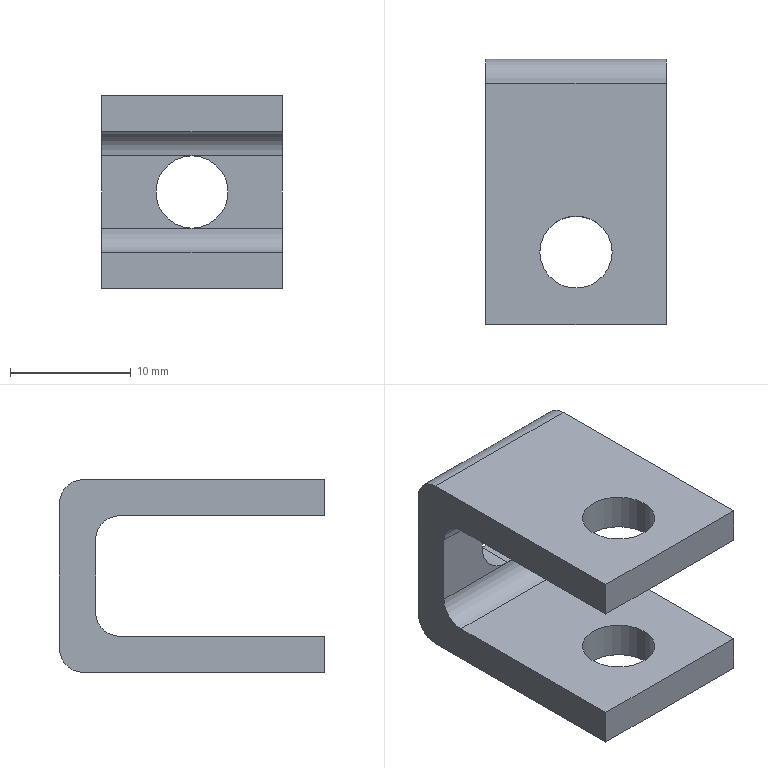Part | SolidWorks | features ICE 2, Extrusion 1, Fillet 1 | 1 solid | 21 faces | box 15 x 22 x 16 mm | volume 2176 mm3 | plane 11 | cylinder 10 | commonest cylinder face diameters 6 x6 4 x4
STEP:
#1=CARTESIAN_POINT('',(0.,13.,-3.));
#2=VERTEX_POINT('',#1);
#3=CARTESIAN_POINT('',(0.,13.,3.));
#4=VERTEX_POINT('',#3);
#5=CARTESIAN_POINT('',(0.,13.,0.));
#6=DIRECTION('',(0.,1.,0.));
#7=DIRECTION('',(0.,0.,1.));
#8=AXIS2_PLACEMENT_3D('',#5,#6,#7);
#9=CIRCLE('',#8,3.);
#10=EDGE_CURVE('',#2,#4,#9,.T.);
#11=ORIENTED_EDGE('',*,*,#10,.F.);
#12=CARTESIAN_POINT('',(0.,16.,-3.));
#13=VERTEX_POINT('',#12);
#14=CARTESIAN_POINT('',(0.,-2.,-3.));
#15=DIRECTION('',(0.,1.,0.));
#16=VECTOR('',#15,1000.);
#17=LINE('',#14,#16);
#18=EDGE_CURVE('',#2,#13,#17,.T.);
#19=ORIENTED_EDGE('',*,*,#18,.T.);
#20=CARTESIAN_POINT('',(0.,16.,3.));
#21=VERTEX_POINT('',#20);
#22=CARTESIAN_POINT('',(0.,16.,0.));
#23=DIRECTION('',(0.,1.,0.));
#24=DIRECTION('',(0.,0.,1.));
#25=AXIS2_PLACEMENT_3D('',#22,#23,#24);
#26=CIRCLE('',#25,3.);
#27=EDGE_CURVE('',#13,#21,#26,.T.);
#28=ORIENTED_EDGE('',*,*,#27,.T.);
#29=CARTESIAN_POINT('',(0.,-2.,3.));
#30=DIRECTION('',(0.,1.,0.));
#31=VECTOR('',#30,1000.);
#32=LINE('',#29,#31);
#33=EDGE_CURVE('',#4,#21,#32,.T.);
#34=ORIENTED_EDGE('',*,*,#33,.F.);
#35=EDGE_LOOP('',(#11,#19,#28,#34));
#36=FACE_OUTER_BOUND('',#35,.T.);
#37=CARTESIAN_POINT('',(0.,-2.,0.));
#38=DIRECTION('',(0.,1.,0.));
#39=DIRECTION('',(0.,0.,1.));
#40=AXIS2_PLACEMENT_3D('',#37,#38,#39);
#41=CYLINDRICAL_SURFACE('',#40,3.);
#42=ADVANCED_FACE('',(#36),#41,.F.);
#43=CARTESIAN_POINT('',(3.,0.,-5.));
#44=VERTEX_POINT('',#43);
#45=CARTESIAN_POINT('',(-3.,0.,-5.));
#46=VERTEX_POINT('',#45);
#47=CARTESIAN_POINT('',(0.,0.,-5.));
#48=DIRECTION('',(0.,0.,-1.));
#49=DIRECTION('',(-1.,0.,0.));
#50=AXIS2_PLACEMENT_3D('',#47,#48,#49);
#51=CIRCLE('',#50,3.);
#52=EDGE_CURVE('',#44,#46,#51,.T.);
#53=ORIENTED_EDGE('',*,*,#52,.F.);
#54=CARTESIAN_POINT('',(3.,0.,-8.));
#55=VERTEX_POINT('',#54);
#56=CARTESIAN_POINT('',(3.,0.,8.));
#57=DIRECTION('',(0.,0.,-1.));
#58=VECTOR('',#57,1000.);
#59=LINE('',#56,#58);
#60=EDGE_CURVE('',#44,#55,#59,.T.);
#61=ORIENTED_EDGE('',*,*,#60,.T.);
#62=CARTESIAN_POINT('',(-3.,0.,-8.));
#63=VERTEX_POINT('',#62);
#64=CARTESIAN_POINT('',(0.,0.,-8.));
#65=DIRECTION('',(0.,0.,1.));
#66=DIRECTION('',(1.,0.,0.));
#67=AXIS2_PLACEMENT_3D('',#64,#65,#66);
#68=CIRCLE('',#67,3.);
#69=EDGE_CURVE('',#63,#55,#68,.T.);
#70=ORIENTED_EDGE('',*,*,#69,.F.);
#71=CARTESIAN_POINT('',(-3.,0.,8.));
#72=DIRECTION('',(0.,0.,-1.));
#73=VECTOR('',#72,1000.);
#74=LINE('',#71,#73);
#75=EDGE_CURVE('',#46,#63,#74,.T.);
#76=ORIENTED_EDGE('',*,*,#75,.F.);
#77=EDGE_LOOP('',(#53,#61,#70,#76));
#78=FACE_OUTER_BOUND('',#77,.T.);
#79=CARTESIAN_POINT('',(0.,0.,8.));
#80=DIRECTION('',(0.,0.,-1.));
#81=DIRECTION('',(-1.,0.,0.));
#82=AXIS2_PLACEMENT_3D('',#79,#80,#81);
#83=CYLINDRICAL_SURFACE('',#82,3.);
#84=ADVANCED_FACE('',(#78),#83,.F.);
#85=CARTESIAN_POINT('',(-3.,0.,8.));
#86=VERTEX_POINT('',#85);
#87=CARTESIAN_POINT('',(3.,0.,8.));
#88=VERTEX_POINT('',#87);
#89=CARTESIAN_POINT('',(0.,0.,8.));
#90=DIRECTION('',(0.,0.,1.));
#91=DIRECTION('',(1.,0.,0.));
#92=AXIS2_PLACEMENT_3D('',#89,#90,#91);
#93=CIRCLE('',#92,3.);
#94=EDGE_CURVE('',#86,#88,#93,.T.);
#95=ORIENTED_EDGE('',*,*,#94,.T.);
#96=CARTESIAN_POINT('',(3.,0.,5.));
#97=VERTEX_POINT('',#96);
#98=CARTESIAN_POINT('',(3.,0.,8.));
#99=DIRECTION('',(0.,0.,-1.));
#100=VECTOR('',#99,1000.);
#101=LINE('',#98,#100);
#102=EDGE_CURVE('',#88,#97,#101,.T.);
#103=ORIENTED_EDGE('',*,*,#102,.T.);
#104=CARTESIAN_POINT('',(-3.,0.,5.));
#105=VERTEX_POINT('',#104);
#106=CARTESIAN_POINT('',(0.,0.,5.));
#107=DIRECTION('',(0.,0.,1.));
#108=DIRECTION('',(1.,0.,0.));
#109=AXIS2_PLACEMENT_3D('',#106,#107,#108);
#110=CIRCLE('',#109,3.);
#111=EDGE_CURVE('',#105,#97,#110,.T.);
#112=ORIENTED_EDGE('',*,*,#111,.F.);
#113=CARTESIAN_POINT('',(-3.,0.,8.));
#114=DIRECTION('',(0.,0.,-1.));
#115=VECTOR('',#114,1000.);
#116=LINE('',#113,#115);
#117=EDGE_CURVE('',#86,#105,#116,.T.);
#118=ORIENTED_EDGE('',*,*,#117,.F.);
#119=EDGE_LOOP('',(#95,#103,#112,#118));
#120=FACE_OUTER_BOUND('',#119,.T.);
#121=CARTESIAN_POINT('',(0.,0.,8.));
#122=DIRECTION('',(0.,0.,-1.));
#123=DIRECTION('',(-1.,0.,0.));
#124=AXIS2_PLACEMENT_3D('',#121,#122,#123);
#125=CYLINDRICAL_SURFACE('',#124,3.);
#126=ADVANCED_FACE('',(#120),#125,.F.);
#127=CARTESIAN_POINT('',(7.5,13.,3.));
#128=VERTEX_POINT('',#127);
#129=CARTESIAN_POINT('',(-7.5,13.,3.));
#130=DIRECTION('',(-1.,0.,0.));
#131=VECTOR('',#130,1000.);
#132=LINE('',#129,#131);
#133=EDGE_CURVE('',#128,#4,#132,.T.);
#134=ORIENTED_EDGE('',*,*,#133,.T.);
#135=CARTESIAN_POINT('',(0.,13.,0.));
#136=DIRECTION('',(0.,1.,0.));
#137=DIRECTION('',(0.,0.,1.));
#138=AXIS2_PLACEMENT_3D('',#135,#136,#137);
#139=CIRCLE('',#138,3.);
#140=EDGE_CURVE('',#4,#2,#139,.T.);
#141=ORIENTED_EDGE('',*,*,#140,.T.);
#142=CARTESIAN_POINT('',(7.5,13.,-3.));
#143=VERTEX_POINT('',#142);
#144=CARTESIAN_POINT('',(7.5,13.,-3.));
#145=DIRECTION('',(1.,0.,0.));
#146=VECTOR('',#145,1000.);
#147=LINE('',#144,#146);
#148=EDGE_CURVE('',#2,#143,#147,.T.);
#149=ORIENTED_EDGE('',*,*,#148,.T.);
#150=CARTESIAN_POINT('',(7.5,13.,5.));
#151=DIRECTION('',(0.,0.,1.));
#152=VECTOR('',#151,1000.);
#153=LINE('',#150,#152);
#154=EDGE_CURVE('',#143,#128,#153,.T.);
#155=ORIENTED_EDGE('',*,*,#154,.T.);
#156=EDGE_LOOP('',(#134,#141,#149,#155));
#157=FACE_OUTER_BOUND('',#156,.T.);
#158=CARTESIAN_POINT('',(-7.5,13.,5.));
#159=DIRECTION('',(0.,1.,0.));
#160=DIRECTION('',(0.,0.,1.));
#161=AXIS2_PLACEMENT_3D('',#158,#159,#160);
#162=PLANE('',#161);
#163=ADVANCED_FACE('',(#157),#162,.F.);
#164=CARTESIAN_POINT('',(-7.5,-6.,8.));
#165=VERTEX_POINT('',#164);
#166=CARTESIAN_POINT('',(-7.5,-6.,5.));
#167=VERTEX_POINT('',#166);
#168=CARTESIAN_POINT('',(-7.5,-6.,8.));
#169=DIRECTION('',(0.,0.,-1.));
#170=VECTOR('',#169,1000.);
#171=LINE('',#168,#170);
#172=EDGE_CURVE('',#165,#167,#171,.T.);
#173=ORIENTED_EDGE('',*,*,#172,.T.);
#174=CARTESIAN_POINT('',(7.5,-6.,5.));
#175=VERTEX_POINT('',#174);
#176=CARTESIAN_POINT('',(-7.5,-6.,5.));
#177=DIRECTION('',(1.,0.,0.));
#178=VECTOR('',#177,1000.);
#179=LINE('',#176,#178);
#180=EDGE_CURVE('',#167,#175,#179,.T.);
#181=ORIENTED_EDGE('',*,*,#180,.T.);
#182=CARTESIAN_POINT('',(7.5,-6.,8.));
#183=VERTEX_POINT('',#182);
#184=CARTESIAN_POINT('',(7.5,-6.,8.));
#185=DIRECTION('',(0.,0.,-1.));
#186=VECTOR('',#185,1000.);
#187=LINE('',#184,#186);
#188=EDGE_CURVE('',#183,#175,#187,.T.);
#189=ORIENTED_EDGE('',*,*,#188,.F.);
#190=CARTESIAN_POINT('',(-7.5,-6.,8.));
#191=DIRECTION('',(1.,0.,0.));
#192=VECTOR('',#191,1000.);
#193=LINE('',#190,#192);
#194=EDGE_CURVE('',#165,#183,#193,.T.);
#195=ORIENTED_EDGE('',*,*,#194,.F.);
#196=EDGE_LOOP('',(#173,#181,#189,#195));
#197=FACE_OUTER_BOUND('',#196,.T.);
#198=CARTESIAN_POINT('',(-7.5,-6.,8.));
#199=DIRECTION('',(0.,1.,0.));
#200=DIRECTION('',(0.,0.,1.));
#201=AXIS2_PLACEMENT_3D('',#198,#199,#200);
#202=PLANE('',#201);
#203=ADVANCED_FACE('',(#197),#202,.F.);
#204=ORIENTED_EDGE('',*,*,#102,.F.);
#205=CARTESIAN_POINT('',(0.,0.,8.));
#206=DIRECTION('',(0.,0.,1.));
#207=DIRECTION('',(1.,0.,0.));
#208=AXIS2_PLACEMENT_3D('',#205,#206,#207);
#209=CIRCLE('',#208,3.);
#210=EDGE_CURVE('',#88,#86,#209,.T.);
#211=ORIENTED_EDGE('',*,*,#210,.T.);
#212=ORIENTED_EDGE('',*,*,#117,.T.);
#213=CARTESIAN_POINT('',(0.,0.,5.));
#214=DIRECTION('',(0.,0.,1.));
#215=DIRECTION('',(1.,0.,0.));
#216=AXIS2_PLACEMENT_3D('',#213,#214,#215);
#217=CIRCLE('',#216,3.);
#218=EDGE_CURVE('',#97,#105,#217,.T.);
#219=ORIENTED_EDGE('',*,*,#218,.F.);
#220=EDGE_LOOP('',(#204,#211,#212,#219));
#221=FACE_OUTER_BOUND('',#220,.T.);
#222=CARTESIAN_POINT('',(0.,0.,8.));
#223=DIRECTION('',(0.,0.,-1.));
#224=DIRECTION('',(-1.,0.,0.));
#225=AXIS2_PLACEMENT_3D('',#222,#223,#224);
#226=CYLINDRICAL_SURFACE('',#225,3.);
#227=ADVANCED_FACE('',(#221),#226,.F.);
#228=CARTESIAN_POINT('',(7.5,14.,8.));
#229=VERTEX_POINT('',#228);
#230=CARTESIAN_POINT('',(7.5,-6.,8.));
#231=DIRECTION('',(0.,1.,0.));
#232=VECTOR('',#231,1000.);
#233=LINE('',#230,#232);
#234=EDGE_CURVE('',#183,#229,#233,.T.);
#235=ORIENTED_EDGE('',*,*,#234,.T.);
#236=CARTESIAN_POINT('',(-7.5,14.,8.));
#237=VERTEX_POINT('',#236);
#238=CARTESIAN_POINT('',(0.,14.,8.));
#239=DIRECTION('',(-1.,0.,0.));
#240=VECTOR('',#239,1000.);
#241=LINE('',#238,#240);
#242=EDGE_CURVE('',#229,#237,#241,.T.);
#243=ORIENTED_EDGE('',*,*,#242,.T.);
#244=CARTESIAN_POINT('',(-7.5,-6.,8.));
#245=DIRECTION('',(0.,-1.,0.));
#246=VECTOR('',#245,1000.);
#247=LINE('',#244,#246);
#248=EDGE_CURVE('',#237,#165,#247,.T.);
#249=ORIENTED_EDGE('',*,*,#248,.T.);
#250=ORIENTED_EDGE('',*,*,#194,.T.);
#251=EDGE_LOOP('',(#235,#243,#249,#250));
#252=FACE_OUTER_BOUND('',#251,.T.);
#253=ORIENTED_EDGE('',*,*,#94,.F.);
#254=ORIENTED_EDGE('',*,*,#210,.F.);
#255=EDGE_LOOP('',(#253,#254));
#256=FACE_BOUND('',#255,.T.);
#257=CARTESIAN_POINT('',(0.,0.,8.));
#258=DIRECTION('',(0.,0.,-1.));
#259=DIRECTION('',(-1.,0.,0.));
#260=AXIS2_PLACEMENT_3D('',#257,#258,#259);
#261=PLANE('',#260);
#262=ADVANCED_FACE('',(#252,#256),#261,.F.);
#263=CARTESIAN_POINT('',(-7.5,14.,-8.));
#264=VERTEX_POINT('',#263);
#265=CARTESIAN_POINT('',(-7.5,-6.,-8.));
#266=VERTEX_POINT('',#265);
#267=CARTESIAN_POINT('',(-7.5,-6.,-8.));
#268=DIRECTION('',(0.,-1.,0.));
#269=VECTOR('',#268,1000.);
#270=LINE('',#267,#269);
#271=EDGE_CURVE('',#264,#266,#270,.T.);
#272=ORIENTED_EDGE('',*,*,#271,.F.);
#273=CARTESIAN_POINT('',(7.5,14.,-8.));
#274=VERTEX_POINT('',#273);
#275=CARTESIAN_POINT('',(7.5,14.,-8.));
#276=DIRECTION('',(1.,0.,0.));
#277=VECTOR('',#276,1000.);
#278=LINE('',#275,#277);
#279=EDGE_CURVE('',#264,#274,#278,.T.);
#280=ORIENTED_EDGE('',*,*,#279,.T.);
#281=CARTESIAN_POINT('',(7.5,-6.,-8.));
#282=VERTEX_POINT('',#281);
#283=CARTESIAN_POINT('',(7.5,-6.,-8.));
#284=DIRECTION('',(0.,1.,0.));
#285=VECTOR('',#284,1000.);
#286=LINE('',#283,#285);
#287=EDGE_CURVE('',#282,#274,#286,.T.);
#288=ORIENTED_EDGE('',*,*,#287,.F.);
#289=CARTESIAN_POINT('',(-7.5,-6.,-8.));
#290=DIRECTION('',(1.,0.,0.));
#291=VECTOR('',#290,1000.);
#292=LINE('',#289,#291);
#293=EDGE_CURVE('',#266,#282,#292,.T.);
#294=ORIENTED_EDGE('',*,*,#293,.F.);
#295=EDGE_LOOP('',(#272,#280,#288,#294));
#296=FACE_OUTER_BOUND('',#295,.T.);
#297=ORIENTED_EDGE('',*,*,#69,.T.);
#298=CARTESIAN_POINT('',(0.,0.,-8.));
#299=DIRECTION('',(0.,0.,1.));
#300=DIRECTION('',(1.,0.,0.));
#301=AXIS2_PLACEMENT_3D('',#298,#299,#300);
#302=CIRCLE('',#301,3.);
#303=EDGE_CURVE('',#55,#63,#302,.T.);
#304=ORIENTED_EDGE('',*,*,#303,.T.);
#305=EDGE_LOOP('',(#297,#304));
#306=FACE_BOUND('',#305,.T.);
#307=CARTESIAN_POINT('',(0.,0.,-8.));
#308=DIRECTION('',(0.,0.,-1.));
#309=DIRECTION('',(-1.,0.,0.));
#310=AXIS2_PLACEMENT_3D('',#307,#308,#309);
#311=PLANE('',#310);
#312=ADVANCED_FACE('',(#296,#306),#311,.T.);
#313=CARTESIAN_POINT('',(-7.5,16.,6.));
#314=VERTEX_POINT('',#313);
#315=CARTESIAN_POINT('',(-7.5,16.,-6.));
#316=VERTEX_POINT('',#315);
#317=CARTESIAN_POINT('',(-7.5,16.,8.));
#318=DIRECTION('',(0.,0.,-1.));
#319=VECTOR('',#318,1000.);
#320=LINE('',#317,#319);
#321=EDGE_CURVE('',#314,#316,#320,.T.);
#322=ORIENTED_EDGE('',*,*,#321,.T.);
#323=CARTESIAN_POINT('',(-7.5,14.,-6.));
#324=DIRECTION('',(-1.,0.,0.));
#325=DIRECTION('',(0.,0.,-1.));
#326=AXIS2_PLACEMENT_3D('',#323,#324,#325);
#327=CIRCLE('',#326,2.);
#328=EDGE_CURVE('',#316,#264,#327,.T.);
#329=ORIENTED_EDGE('',*,*,#328,.T.);
#330=ORIENTED_EDGE('',*,*,#271,.T.);
#331=CARTESIAN_POINT('',(-7.5,-6.,-5.));
#332=VERTEX_POINT('',#331);
#333=CARTESIAN_POINT('',(-7.5,-6.,8.));
#334=DIRECTION('',(0.,0.,-1.));
#335=VECTOR('',#334,1000.);
#336=LINE('',#333,#335);
#337=EDGE_CURVE('',#332,#266,#336,.T.);
#338=ORIENTED_EDGE('',*,*,#337,.F.);
#339=CARTESIAN_POINT('',(-7.5,11.,-5.));
#340=VERTEX_POINT('',#339);
#341=CARTESIAN_POINT('',(-7.5,-6.,-5.));
#342=DIRECTION('',(0.,1.,0.));
#343=VECTOR('',#342,1000.);
#344=LINE('',#341,#343);
#345=EDGE_CURVE('',#332,#340,#344,.T.);
#346=ORIENTED_EDGE('',*,*,#345,.T.);
#347=CARTESIAN_POINT('',(-7.5,13.,-3.));
#348=VERTEX_POINT('',#347);
#349=CARTESIAN_POINT('',(-7.5,11.,-3.));
#350=DIRECTION('',(1.,0.,0.));
#351=DIRECTION('',(0.,0.,-1.));
#352=AXIS2_PLACEMENT_3D('',#349,#350,#351);
#353=CIRCLE('',#352,2.);
#354=EDGE_CURVE('',#340,#348,#353,.T.);
#355=ORIENTED_EDGE('',*,*,#354,.T.);
#356=CARTESIAN_POINT('',(-7.5,13.,3.));
#357=VERTEX_POINT('',#356);
#358=CARTESIAN_POINT('',(-7.5,13.,5.));
#359=DIRECTION('',(0.,0.,1.));
#360=VECTOR('',#359,1000.);
#361=LINE('',#358,#360);
#362=EDGE_CURVE('',#348,#357,#361,.T.);
#363=ORIENTED_EDGE('',*,*,#362,.T.);
#364=CARTESIAN_POINT('',(-7.5,11.,5.));
#365=VERTEX_POINT('',#364);
#366=CARTESIAN_POINT('',(-7.5,11.,3.));
#367=DIRECTION('',(1.,0.,0.));
#368=DIRECTION('',(0.,0.,-1.));
#369=AXIS2_PLACEMENT_3D('',#366,#367,#368);
#370=CIRCLE('',#369,2.);
#371=EDGE_CURVE('',#357,#365,#370,.T.);
#372=ORIENTED_EDGE('',*,*,#371,.T.);
#373=CARTESIAN_POINT('',(-7.5,-6.,5.));
#374=DIRECTION('',(0.,-1.,0.));
#375=VECTOR('',#374,1000.);
#376=LINE('',#373,#375);
#377=EDGE_CURVE('',#365,#167,#376,.T.);
#378=ORIENTED_EDGE('',*,*,#377,.T.);
#379=ORIENTED_EDGE('',*,*,#172,.F.);
#380=ORIENTED_EDGE('',*,*,#248,.F.);
#381=CARTESIAN_POINT('',(-7.5,14.,6.));
#382=DIRECTION('',(-1.,0.,0.));
#383=DIRECTION('',(0.,0.,-1.));
#384=AXIS2_PLACEMENT_3D('',#381,#382,#383);
#385=CIRCLE('',#384,2.);
#386=EDGE_CURVE('',#237,#314,#385,.T.);
#387=ORIENTED_EDGE('',*,*,#386,.T.);
#388=EDGE_LOOP('',(#322,#329,#330,#338,#346,#355,#363,#372,#378,#379,#380,#387));
#389=FACE_OUTER_BOUND('',#388,.T.);
#390=CARTESIAN_POINT('',(-7.5,-6.,8.));
#391=DIRECTION('',(1.,0.,0.));
#392=DIRECTION('',(0.,0.,-1.));
#393=AXIS2_PLACEMENT_3D('',#390,#391,#392);
#394=PLANE('',#393);
#395=ADVANCED_FACE('',(#389),#394,.F.);
#396=CARTESIAN_POINT('',(7.5,-6.,-5.));
#397=VERTEX_POINT('',#396);
#398=CARTESIAN_POINT('',(7.5,-6.,8.));
#399=DIRECTION('',(0.,0.,-1.));
#400=VECTOR('',#399,1000.);
#401=LINE('',#398,#400);
#402=EDGE_CURVE('',#397,#282,#401,.T.);
#403=ORIENTED_EDGE('',*,*,#402,.F.);
#404=CARTESIAN_POINT('',(-7.5,-6.,-5.));
#405=DIRECTION('',(1.,0.,0.));
#406=VECTOR('',#405,1000.);
#407=LINE('',#404,#406);
#408=EDGE_CURVE('',#332,#397,#407,.T.);
#409=ORIENTED_EDGE('',*,*,#408,.F.);
#410=ORIENTED_EDGE('',*,*,#337,.T.);
#411=ORIENTED_EDGE('',*,*,#293,.T.);
#412=EDGE_LOOP('',(#403,#409,#410,#411));
#413=FACE_OUTER_BOUND('',#412,.T.);
#414=CARTESIAN_POINT('',(-7.5,-6.,8.));
#415=DIRECTION('',(0.,1.,0.));
#416=DIRECTION('',(0.,0.,1.));
#417=AXIS2_PLACEMENT_3D('',#414,#415,#416);
#418=PLANE('',#417);
#419=ADVANCED_FACE('',(#413),#418,.F.);
#420=ORIENTED_EDGE('',*,*,#287,.T.);
#421=CARTESIAN_POINT('',(7.5,16.,-6.));
#422=VERTEX_POINT('',#421);
#423=CARTESIAN_POINT('',(7.5,14.,-6.));
#424=DIRECTION('',(1.,0.,0.));
#425=DIRECTION('',(0.,0.,1.));
#426=AXIS2_PLACEMENT_3D('',#423,#424,#425);
#427=CIRCLE('',#426,2.);
#428=EDGE_CURVE('',#274,#422,#427,.T.);
#429=ORIENTED_EDGE('',*,*,#428,.T.);
#430=CARTESIAN_POINT('',(7.5,16.,6.));
#431=VERTEX_POINT('',#430);
#432=CARTESIAN_POINT('',(7.5,16.,8.));
#433=DIRECTION('',(0.,0.,-1.));
#434=VECTOR('',#433,1000.);
#435=LINE('',#432,#434);
#436=EDGE_CURVE('',#431,#422,#435,.T.);
#437=ORIENTED_EDGE('',*,*,#436,.F.);
#438=CARTESIAN_POINT('',(7.5,14.,6.));
#439=DIRECTION('',(1.,0.,0.));
#440=DIRECTION('',(0.,0.,1.));
#441=AXIS2_PLACEMENT_3D('',#438,#439,#440);
#442=CIRCLE('',#441,2.);
#443=EDGE_CURVE('',#431,#229,#442,.T.);
#444=ORIENTED_EDGE('',*,*,#443,.T.);
#445=ORIENTED_EDGE('',*,*,#234,.F.);
#446=ORIENTED_EDGE('',*,*,#188,.T.);
#447=CARTESIAN_POINT('',(7.5,11.,5.));
#448=VERTEX_POINT('',#447);
#449=CARTESIAN_POINT('',(7.5,-6.,5.));
#450=DIRECTION('',(0.,-1.,0.));
#451=VECTOR('',#450,1000.);
#452=LINE('',#449,#451);
#453=EDGE_CURVE('',#448,#175,#452,.T.);
#454=ORIENTED_EDGE('',*,*,#453,.F.);
#455=CARTESIAN_POINT('',(7.5,11.,3.));
#456=DIRECTION('',(-1.,0.,0.));
#457=DIRECTION('',(0.,0.,1.));
#458=AXIS2_PLACEMENT_3D('',#455,#456,#457);
#459=CIRCLE('',#458,2.);
#460=EDGE_CURVE('',#448,#128,#459,.T.);
#461=ORIENTED_EDGE('',*,*,#460,.T.);
#462=ORIENTED_EDGE('',*,*,#154,.F.);
#463=CARTESIAN_POINT('',(7.5,11.,-5.));
#464=VERTEX_POINT('',#463);
#465=CARTESIAN_POINT('',(7.5,11.,-3.));
#466=DIRECTION('',(-1.,0.,0.));
#467=DIRECTION('',(0.,0.,1.));
#468=AXIS2_PLACEMENT_3D('',#465,#466,#467);
#469=CIRCLE('',#468,2.);
#470=EDGE_CURVE('',#143,#464,#469,.T.);
#471=ORIENTED_EDGE('',*,*,#470,.T.);
#472=CARTESIAN_POINT('',(7.5,-6.,-5.));
#473=DIRECTION('',(0.,1.,0.));
#474=VECTOR('',#473,1000.);
#475=LINE('',#472,#474);
#476=EDGE_CURVE('',#397,#464,#475,.T.);
#477=ORIENTED_EDGE('',*,*,#476,.F.);
#478=ORIENTED_EDGE('',*,*,#402,.T.);
#479=EDGE_LOOP('',(#420,#429,#437,#444,#445,#446,#454,#461,#462,#471,#477,#478));
#480=FACE_OUTER_BOUND('',#479,.T.);
#481=CARTESIAN_POINT('',(7.5,-6.,8.));
#482=DIRECTION('',(-1.,0.,0.));
#483=DIRECTION('',(0.,0.,1.));
#484=AXIS2_PLACEMENT_3D('',#481,#482,#483);
#485=PLANE('',#484);
#486=ADVANCED_FACE('',(#480),#485,.F.);
#487=CARTESIAN_POINT('',(0.,16.,0.));
#488=DIRECTION('',(0.,1.,0.));
#489=DIRECTION('',(0.,0.,1.));
#490=AXIS2_PLACEMENT_3D('',#487,#488,#489);
#491=CIRCLE('',#490,3.);
#492=EDGE_CURVE('',#21,#13,#491,.T.);
#493=ORIENTED_EDGE('',*,*,#492,.F.);
#494=ORIENTED_EDGE('',*,*,#27,.F.);
#495=EDGE_LOOP('',(#493,#494));
#496=FACE_BOUND('',#495,.T.);
#497=ORIENTED_EDGE('',*,*,#436,.T.);
#498=CARTESIAN_POINT('',(-7.5,16.,-6.));
#499=DIRECTION('',(-1.,0.,0.));
#500=VECTOR('',#499,1000.);
#501=LINE('',#498,#500);
#502=EDGE_CURVE('',#422,#316,#501,.T.);
#503=ORIENTED_EDGE('',*,*,#502,.T.);
#504=ORIENTED_EDGE('',*,*,#321,.F.);
#505=CARTESIAN_POINT('',(-7.5,16.,6.));
#506=DIRECTION('',(1.,0.,0.));
#507=VECTOR('',#506,1000.);
#508=LINE('',#505,#507);
#509=EDGE_CURVE('',#314,#431,#508,.T.);
#510=ORIENTED_EDGE('',*,*,#509,.T.);
#511=EDGE_LOOP('',(#497,#503,#504,#510));
#512=FACE_OUTER_BOUND('',#511,.T.);
#513=CARTESIAN_POINT('',(-7.5,16.,8.));
#514=DIRECTION('',(0.,-1.,0.));
#515=DIRECTION('',(0.,0.,-1.));
#516=AXIS2_PLACEMENT_3D('',#513,#514,#515);
#517=PLANE('',#516);
#518=ADVANCED_FACE('',(#496,#512),#517,.F.);
#519=ORIENTED_EDGE('',*,*,#60,.F.);
#520=CARTESIAN_POINT('',(0.,0.,-5.));
#521=DIRECTION('',(0.,0.,-1.));
#522=DIRECTION('',(-1.,0.,0.));
#523=AXIS2_PLACEMENT_3D('',#520,#521,#522);
#524=CIRCLE('',#523,3.);
#525=EDGE_CURVE('',#46,#44,#524,.T.);
#526=ORIENTED_EDGE('',*,*,#525,.F.);
#527=ORIENTED_EDGE('',*,*,#75,.T.);
#528=ORIENTED_EDGE('',*,*,#303,.F.);
#529=EDGE_LOOP('',(#519,#526,#527,#528));
#530=FACE_OUTER_BOUND('',#529,.T.);
#531=CARTESIAN_POINT('',(0.,0.,8.));
#532=DIRECTION('',(0.,0.,-1.));
#533=DIRECTION('',(-1.,0.,0.));
#534=AXIS2_PLACEMENT_3D('',#531,#532,#533);
#535=CYLINDRICAL_SURFACE('',#534,3.);
#536=ADVANCED_FACE('',(#530),#535,.F.);
#537=ORIENTED_EDGE('',*,*,#111,.T.);
#538=ORIENTED_EDGE('',*,*,#218,.T.);
#539=EDGE_LOOP('',(#537,#538));
#540=FACE_BOUND('',#539,.T.);
#541=ORIENTED_EDGE('',*,*,#377,.F.);
#542=CARTESIAN_POINT('',(7.5,11.,5.));
#543=DIRECTION('',(1.,0.,0.));
#544=VECTOR('',#543,1000.);
#545=LINE('',#542,#544);
#546=EDGE_CURVE('',#365,#448,#545,.T.);
#547=ORIENTED_EDGE('',*,*,#546,.T.);
#548=ORIENTED_EDGE('',*,*,#453,.T.);
#549=ORIENTED_EDGE('',*,*,#180,.F.);
#550=EDGE_LOOP('',(#541,#547,#548,#549));
#551=FACE_OUTER_BOUND('',#550,.T.);
#552=CARTESIAN_POINT('',(-7.5,-6.,5.));
#553=DIRECTION('',(0.,0.,1.));
#554=DIRECTION('',(1.,0.,0.));
#555=AXIS2_PLACEMENT_3D('',#552,#553,#554);
#556=PLANE('',#555);
#557=ADVANCED_FACE('',(#540,#551),#556,.F.);
#558=CARTESIAN_POINT('',(7.5,13.,-3.));
#559=DIRECTION('',(1.,0.,0.));
#560=VECTOR('',#559,1000.);
#561=LINE('',#558,#560);
#562=EDGE_CURVE('',#348,#2,#561,.T.);
#563=ORIENTED_EDGE('',*,*,#562,.T.);
#564=ORIENTED_EDGE('',*,*,#10,.T.);
#565=CARTESIAN_POINT('',(-7.5,13.,3.));
#566=DIRECTION('',(-1.,0.,0.));
#567=VECTOR('',#566,1000.);
#568=LINE('',#565,#567);
#569=EDGE_CURVE('',#4,#357,#568,.T.);
#570=ORIENTED_EDGE('',*,*,#569,.T.);
#571=ORIENTED_EDGE('',*,*,#362,.F.);
#572=EDGE_LOOP('',(#563,#564,#570,#571));
#573=FACE_OUTER_BOUND('',#572,.T.);
#574=CARTESIAN_POINT('',(-7.5,13.,5.));
#575=DIRECTION('',(0.,1.,0.));
#576=DIRECTION('',(0.,0.,1.));
#577=AXIS2_PLACEMENT_3D('',#574,#575,#576);
#578=PLANE('',#577);
#579=ADVANCED_FACE('',(#573),#578,.F.);
#580=ORIENTED_EDGE('',*,*,#525,.T.);
#581=ORIENTED_EDGE('',*,*,#52,.T.);
#582=EDGE_LOOP('',(#580,#581));
#583=FACE_BOUND('',#582,.T.);
#584=ORIENTED_EDGE('',*,*,#476,.T.);
#585=CARTESIAN_POINT('',(-7.5,11.,-5.));
#586=DIRECTION('',(-1.,0.,0.));
#587=VECTOR('',#586,1000.);
#588=LINE('',#585,#587);
#589=EDGE_CURVE('',#464,#340,#588,.T.);
#590=ORIENTED_EDGE('',*,*,#589,.T.);
#591=ORIENTED_EDGE('',*,*,#345,.F.);
#592=ORIENTED_EDGE('',*,*,#408,.T.);
#593=EDGE_LOOP('',(#584,#590,#591,#592));
#594=FACE_OUTER_BOUND('',#593,.T.);
#595=CARTESIAN_POINT('',(-7.5,-6.,-5.));
#596=DIRECTION('',(0.,0.,-1.));
#597=DIRECTION('',(-1.,0.,0.));
#598=AXIS2_PLACEMENT_3D('',#595,#596,#597);
#599=PLANE('',#598);
#600=ADVANCED_FACE('',(#583,#594),#599,.F.);
#601=ORIENTED_EDGE('',*,*,#354,.F.);
#602=ORIENTED_EDGE('',*,*,#589,.F.);
#603=ORIENTED_EDGE('',*,*,#470,.F.);
#604=ORIENTED_EDGE('',*,*,#148,.F.);
#605=ORIENTED_EDGE('',*,*,#562,.F.);
#606=EDGE_LOOP('',(#601,#602,#603,#604,#605));
#607=FACE_OUTER_BOUND('',#606,.T.);
#608=CARTESIAN_POINT('',(-7.5,11.,-3.));
#609=DIRECTION('',(-1.,0.,0.));
#610=DIRECTION('',(0.,0.,1.));
#611=AXIS2_PLACEMENT_3D('',#608,#609,#610);
#612=CYLINDRICAL_SURFACE('',#611,2.);
#613=ADVANCED_FACE('',(#607),#612,.F.);
#614=ORIENTED_EDGE('',*,*,#428,.F.);
#615=ORIENTED_EDGE('',*,*,#279,.F.);
#616=ORIENTED_EDGE('',*,*,#328,.F.);
#617=ORIENTED_EDGE('',*,*,#502,.F.);
#618=EDGE_LOOP('',(#614,#615,#616,#617));
#619=FACE_OUTER_BOUND('',#618,.T.);
#620=CARTESIAN_POINT('',(-7.5,14.,-6.));
#621=DIRECTION('',(1.,0.,0.));
#622=DIRECTION('',(0.,0.,-1.));
#623=AXIS2_PLACEMENT_3D('',#620,#621,#622);
#624=CYLINDRICAL_SURFACE('',#623,2.);
#625=ADVANCED_FACE('',(#619),#624,.T.);
#626=ORIENTED_EDGE('',*,*,#443,.F.);
#627=ORIENTED_EDGE('',*,*,#509,.F.);
#628=ORIENTED_EDGE('',*,*,#386,.F.);
#629=ORIENTED_EDGE('',*,*,#242,.F.);
#630=EDGE_LOOP('',(#626,#627,#628,#629));
#631=FACE_OUTER_BOUND('',#630,.T.);
#632=CARTESIAN_POINT('',(0.,14.,6.));
#633=DIRECTION('',(-1.,0.,0.));
#634=DIRECTION('',(0.,0.,1.));
#635=AXIS2_PLACEMENT_3D('',#632,#633,#634);
#636=CYLINDRICAL_SURFACE('',#635,2.);
#637=ADVANCED_FACE('',(#631),#636,.T.);
#638=ORIENTED_EDGE('',*,*,#371,.F.);
#639=ORIENTED_EDGE('',*,*,#569,.F.);
#640=ORIENTED_EDGE('',*,*,#133,.F.);
#641=ORIENTED_EDGE('',*,*,#460,.F.);
#642=ORIENTED_EDGE('',*,*,#546,.F.);
#643=EDGE_LOOP('',(#638,#639,#640,#641,#642));
#644=FACE_OUTER_BOUND('',#643,.T.);
#645=CARTESIAN_POINT('',(-7.5,11.,3.));
#646=DIRECTION('',(-1.,0.,0.));
#647=DIRECTION('',(0.,0.,1.));
#648=AXIS2_PLACEMENT_3D('',#645,#646,#647);
#649=CYLINDRICAL_SURFACE('',#648,2.);
#650=ADVANCED_FACE('',(#644),#649,.F.);
#651=ORIENTED_EDGE('',*,*,#18,.F.);
#652=ORIENTED_EDGE('',*,*,#140,.F.);
#653=ORIENTED_EDGE('',*,*,#33,.T.);
#654=ORIENTED_EDGE('',*,*,#492,.T.);
#655=EDGE_LOOP('',(#651,#652,#653,#654));
#656=FACE_OUTER_BOUND('',#655,.T.);
#657=CARTESIAN_POINT('',(0.,-2.,0.));
#658=DIRECTION('',(0.,1.,0.));
#659=DIRECTION('',(0.,0.,1.));
#660=AXIS2_PLACEMENT_3D('',#657,#658,#659);
#661=CYLINDRICAL_SURFACE('',#660,3.);
#662=ADVANCED_FACE('',(#656),#661,.F.);
#663=CLOSED_SHELL('',(#42,#84,#126,#163,#203,#227,#262,#312,#395,#419,#486,#518,#536,#557,#579,#600,#613,#625,#637,#650,#662));
#664=MANIFOLD_SOLID_BREP('',#663);
#665=CARTESIAN_POINT('',(0.,0.,0.));
#666=DIRECTION('',(0.,0.,1.));
#667=DIRECTION('',(1.,0.,0.));
#668=AXIS2_PLACEMENT_3D('',#665,#666,#667);
#669=(LENGTH_UNIT()NAMED_UNIT(*)SI_UNIT(.MILLI.,.METRE.));
#670=UNCERTAINTY_MEASURE_WITH_UNIT(LENGTH_MEASURE(0.00001),#669,'','');
#671=(NAMED_UNIT(*)PLANE_ANGLE_UNIT()SI_UNIT($,.RADIAN.));
#672=(NAMED_UNIT(*)SI_UNIT($,.STERADIAN.)SOLID_ANGLE_UNIT());
#673=(GEOMETRIC_REPRESENTATION_CONTEXT(3)GLOBAL_UNCERTAINTY_ASSIGNED_CONTEXT((#670))GLOBAL_UNIT_ASSIGNED_CONTEXT((#669,#671,#672))REPRESENTATION_CONTEXT('',''));
#674=ADVANCED_BREP_SHAPE_REPRESENTATION('',(#664,#668),#673);